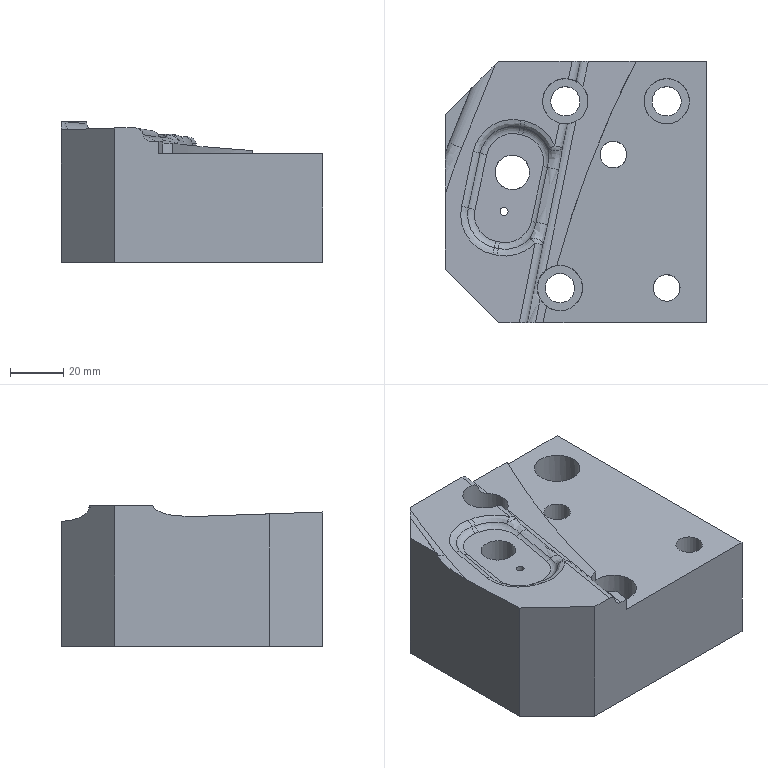Part | NX | features solid 2 | 1 solid | 59 faces | box 98.003 x 98 x 52.792 mm | volume 348992 mm3 | cylinder 20 | plane 18 | spline 12 | torus 7 | sphere 2 | commonest cylinder face diameters 6 x7 10 x3 11 x3 17 x3 3 x1 13 x1